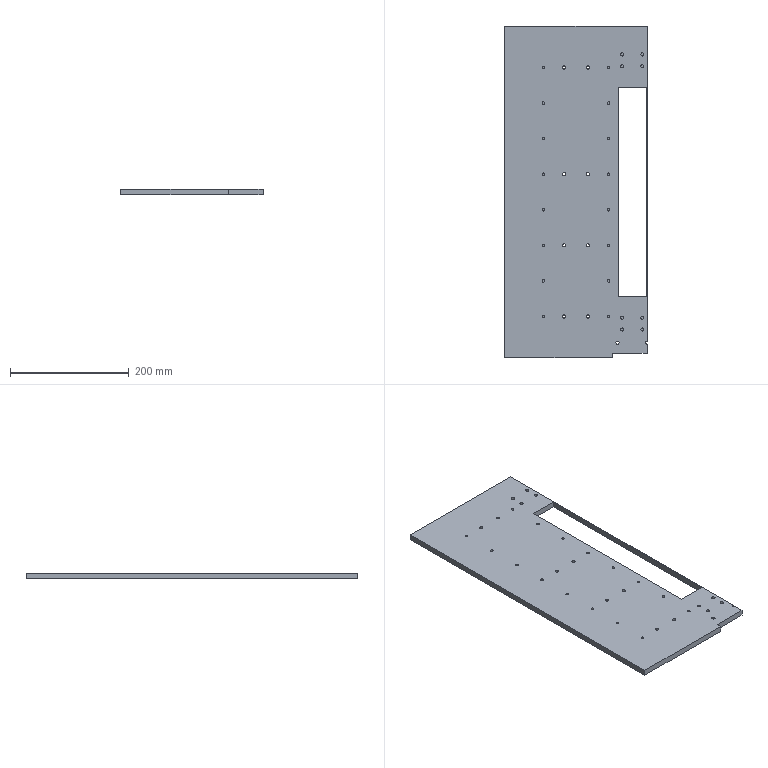Part | SolidWorks | features BaseBody 1 | 1 solid | 104 faces | box 240 x 560 x 10 mm | volume 1164432 mm3 | cylinder 67 | plane 37 | commonest cylinder face diameters 5.3 x35 4.3 x32